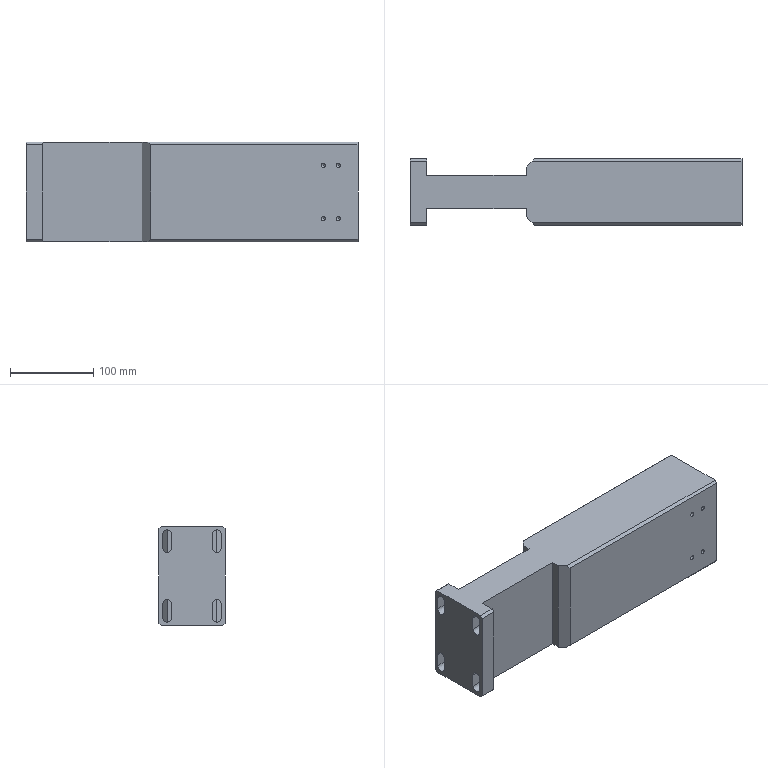Part | 1 solid | 70 faces | box 400 x 80 x 120 mm | volume 3219056 mm3 | plane 32 | cylinder 23 | cone 15 | commonest cylinder face diameters 5 x8 11 x8 6.8 x4 3.3 x3